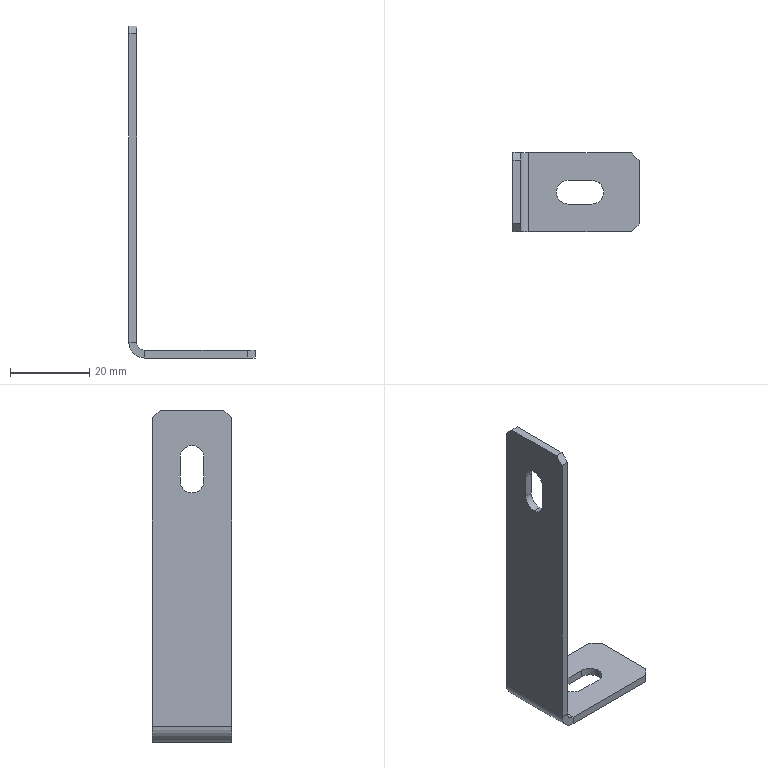Part | NX | features BREP 1 | 1 solid | 28 faces | box 32 x 20 x 84 mm | volume 4235 mm3 | plane 20 | cylinder 8 | commonest cylinder face diameters 6 x6 4 x1 8 x1
STEP:
#1=CARTESIAN_POINT('',(-2.,10.,-2.));
#2=VERTEX_POINT('',#1);
#3=CARTESIAN_POINT('',(0.,8.,-2.));
#4=VERTEX_POINT('',#3);
#5=CARTESIAN_POINT('',(0.,8.,-2.));
#6=DIRECTION('',(0.7071,-0.7071,0.));
#7=VECTOR('',#6,1000.);
#8=LINE('',#5,#7);
#9=EDGE_CURVE('',#2,#4,#8,.T.);
#10=ORIENTED_EDGE('',*,*,#9,.F.);
#11=CARTESIAN_POINT('',(-2.,10.,0.));
#12=VERTEX_POINT('',#11);
#13=CARTESIAN_POINT('',(-2.,10.,-2.));
#14=DIRECTION('',(0.,0.,-1.));
#15=VECTOR('',#14,1000.);
#16=LINE('',#13,#15);
#17=EDGE_CURVE('',#12,#2,#16,.T.);
#18=ORIENTED_EDGE('',*,*,#17,.F.);
#19=CARTESIAN_POINT('',(0.,8.,0.));
#20=VERTEX_POINT('',#19);
#21=CARTESIAN_POINT('',(-1.,9.,0.));
#22=DIRECTION('',(-0.7071,0.7071,0.));
#23=VECTOR('',#22,1000.);
#24=LINE('',#21,#23);
#25=EDGE_CURVE('',#20,#12,#24,.T.);
#26=ORIENTED_EDGE('',*,*,#25,.F.);
#27=CARTESIAN_POINT('',(0.,8.,0.));
#28=DIRECTION('',(0.,0.,1.));
#29=VECTOR('',#28,1000.);
#30=LINE('',#27,#29);
#31=EDGE_CURVE('',#4,#20,#30,.T.);
#32=ORIENTED_EDGE('',*,*,#31,.F.);
#33=EDGE_LOOP('',(#10,#18,#26,#32));
#34=FACE_BOUND('',#33,.T.);
#35=CARTESIAN_POINT('',(0.,8.,-2.));
#36=DIRECTION('',(0.7071,0.7071,0.));
#37=DIRECTION('',(0.,0.,-1.));
#38=AXIS2_PLACEMENT_3D('',#35,#36,#37);
#39=PLANE('',#38);
#40=ADVANCED_FACE('',(#34),#39,.T.);
#41=CARTESIAN_POINT('',(-30.,10.,80.));
#42=VERTEX_POINT('',#41);
#43=CARTESIAN_POINT('',(-30.,8.,82.));
#44=VERTEX_POINT('',#43);
#45=CARTESIAN_POINT('',(-30.,50.,40.));
#46=DIRECTION('',(0.,-0.7071,0.7071));
#47=VECTOR('',#46,1000.);
#48=LINE('',#45,#47);
#49=EDGE_CURVE('',#42,#44,#48,.T.);
#50=ORIENTED_EDGE('',*,*,#49,.F.);
#51=CARTESIAN_POINT('',(-32.,10.,80.));
#52=VERTEX_POINT('',#51);
#53=CARTESIAN_POINT('',(-28.,10.,80.));
#54=DIRECTION('',(1.,0.,0.));
#55=VECTOR('',#54,1000.);
#56=LINE('',#53,#55);
#57=EDGE_CURVE('',#52,#42,#56,.T.);
#58=ORIENTED_EDGE('',*,*,#57,.F.);
#59=CARTESIAN_POINT('',(-32.,8.,82.));
#60=VERTEX_POINT('',#59);
#61=CARTESIAN_POINT('',(-32.,8.,82.));
#62=DIRECTION('',(0.,0.7071,-0.7071));
#63=VECTOR('',#62,1000.);
#64=LINE('',#61,#63);
#65=EDGE_CURVE('',#60,#52,#64,.T.);
#66=ORIENTED_EDGE('',*,*,#65,.F.);
#67=CARTESIAN_POINT('',(-30.,8.,82.));
#68=DIRECTION('',(-1.,0.,0.));
#69=VECTOR('',#68,1000.);
#70=LINE('',#67,#69);
#71=EDGE_CURVE('',#44,#60,#70,.T.);
#72=ORIENTED_EDGE('',*,*,#71,.F.);
#73=EDGE_LOOP('',(#50,#58,#66,#72));
#74=FACE_BOUND('',#73,.T.);
#75=CARTESIAN_POINT('',(-30.,8.,82.));
#76=DIRECTION('',(0.,-0.7071,-0.7071));
#77=DIRECTION('',(-1.,0.,0.));
#78=AXIS2_PLACEMENT_3D('',#75,#76,#77);
#79=PLANE('',#78);
#80=ADVANCED_FACE('',(#74),#79,.F.);
#81=CARTESIAN_POINT('',(0.,-8.,-2.));
#82=VERTEX_POINT('',#81);
#83=CARTESIAN_POINT('',(-2.,-10.,-2.));
#84=VERTEX_POINT('',#83);
#85=CARTESIAN_POINT('',(-2.,-10.,-2.));
#86=DIRECTION('',(-0.7071,-0.7071,0.));
#87=VECTOR('',#86,1000.);
#88=LINE('',#85,#87);
#89=EDGE_CURVE('',#82,#84,#88,.T.);
#90=ORIENTED_EDGE('',*,*,#89,.F.);
#91=CARTESIAN_POINT('',(0.,-8.,0.));
#92=VERTEX_POINT('',#91);
#93=CARTESIAN_POINT('',(0.,-8.,-2.));
#94=DIRECTION('',(0.,0.,-1.));
#95=VECTOR('',#94,1000.);
#96=LINE('',#93,#95);
#97=EDGE_CURVE('',#92,#82,#96,.T.);
#98=ORIENTED_EDGE('',*,*,#97,.F.);
#99=CARTESIAN_POINT('',(-2.,-10.,0.));
#100=VERTEX_POINT('',#99);
#101=CARTESIAN_POINT('',(9.,1.,0.));
#102=DIRECTION('',(0.7071,0.7071,0.));
#103=VECTOR('',#102,1000.);
#104=LINE('',#101,#103);
#105=EDGE_CURVE('',#100,#92,#104,.T.);
#106=ORIENTED_EDGE('',*,*,#105,.F.);
#107=CARTESIAN_POINT('',(-2.,-10.,2.));
#108=DIRECTION('',(0.,0.,1.));
#109=VECTOR('',#108,1000.);
#110=LINE('',#107,#109);
#111=EDGE_CURVE('',#84,#100,#110,.T.);
#112=ORIENTED_EDGE('',*,*,#111,.F.);
#113=EDGE_LOOP('',(#90,#98,#106,#112));
#114=FACE_BOUND('',#113,.T.);
#115=CARTESIAN_POINT('',(-2.,-10.,2.));
#116=DIRECTION('',(-0.7071,0.7071,0.));
#117=DIRECTION('',(0.,0.,1.));
#118=AXIS2_PLACEMENT_3D('',#115,#116,#117);
#119=PLANE('',#118);
#120=ADVANCED_FACE('',(#114),#119,.F.);
#121=CARTESIAN_POINT('',(-30.,-8.,82.));
#122=VERTEX_POINT('',#121);
#123=CARTESIAN_POINT('',(-30.,-10.,80.));
#124=VERTEX_POINT('',#123);
#125=CARTESIAN_POINT('',(-30.,-40.,50.));
#126=DIRECTION('',(0.,-0.7071,-0.7071));
#127=VECTOR('',#126,1000.);
#128=LINE('',#125,#127);
#129=EDGE_CURVE('',#122,#124,#128,.T.);
#130=ORIENTED_EDGE('',*,*,#129,.F.);
#131=CARTESIAN_POINT('',(-32.,-8.,82.));
#132=VERTEX_POINT('',#131);
#133=CARTESIAN_POINT('',(-30.,-8.,82.));
#134=DIRECTION('',(1.,0.,0.));
#135=VECTOR('',#134,1000.);
#136=LINE('',#133,#135);
#137=EDGE_CURVE('',#132,#122,#136,.T.);
#138=ORIENTED_EDGE('',*,*,#137,.F.);
#139=CARTESIAN_POINT('',(-32.,-10.,80.));
#140=VERTEX_POINT('',#139);
#141=CARTESIAN_POINT('',(-32.,-10.,80.));
#142=DIRECTION('',(0.,0.7071,0.7071));
#143=VECTOR('',#142,1000.);
#144=LINE('',#141,#143);
#145=EDGE_CURVE('',#140,#132,#144,.T.);
#146=ORIENTED_EDGE('',*,*,#145,.F.);
#147=CARTESIAN_POINT('',(-28.,-10.,80.));
#148=DIRECTION('',(-1.,0.,0.));
#149=VECTOR('',#148,1000.);
#150=LINE('',#147,#149);
#151=EDGE_CURVE('',#124,#140,#150,.T.);
#152=ORIENTED_EDGE('',*,*,#151,.F.);
#153=EDGE_LOOP('',(#130,#138,#146,#152));
#154=FACE_BOUND('',#153,.T.);
#155=CARTESIAN_POINT('',(-28.,-10.,80.));
#156=DIRECTION('',(0.,0.7071,-0.7071));
#157=DIRECTION('',(-1.,0.,0.));
#158=AXIS2_PLACEMENT_3D('',#155,#156,#157);
#159=PLANE('',#158);
#160=ADVANCED_FACE('',(#154),#159,.F.);
#161=CARTESIAN_POINT('',(-18.,-3.,0.));
#162=VERTEX_POINT('',#161);
#163=CARTESIAN_POINT('',(-12.,-3.,0.));
#164=VERTEX_POINT('',#163);
#165=CARTESIAN_POINT('',(-18.,-3.,0.));
#166=DIRECTION('',(1.,0.,0.));
#167=VECTOR('',#166,1000.);
#168=LINE('',#165,#167);
#169=EDGE_CURVE('',#162,#164,#168,.T.);
#170=ORIENTED_EDGE('',*,*,#169,.T.);
#171=CARTESIAN_POINT('',(-12.,-3.,-2.));
#172=VERTEX_POINT('',#171);
#173=CARTESIAN_POINT('',(-12.,-3.,-2.));
#174=DIRECTION('',(0.,0.,1.));
#175=VECTOR('',#174,1000.);
#176=LINE('',#173,#175);
#177=EDGE_CURVE('',#172,#164,#176,.T.);
#178=ORIENTED_EDGE('',*,*,#177,.F.);
#179=CARTESIAN_POINT('',(-18.,-3.,-2.));
#180=VERTEX_POINT('',#179);
#181=CARTESIAN_POINT('',(-18.,-3.,-2.));
#182=DIRECTION('',(1.,0.,0.));
#183=VECTOR('',#182,1000.);
#184=LINE('',#181,#183);
#185=EDGE_CURVE('',#180,#172,#184,.T.);
#186=ORIENTED_EDGE('',*,*,#185,.F.);
#187=CARTESIAN_POINT('',(-18.,-3.,-2.));
#188=DIRECTION('',(0.,0.,1.));
#189=VECTOR('',#188,1000.);
#190=LINE('',#187,#189);
#191=EDGE_CURVE('',#180,#162,#190,.T.);
#192=ORIENTED_EDGE('',*,*,#191,.T.);
#193=EDGE_LOOP('',(#170,#178,#186,#192));
#194=FACE_BOUND('',#193,.T.);
#195=CARTESIAN_POINT('',(-18.,-3.,-2.));
#196=DIRECTION('',(0.,-1.,0.));
#197=DIRECTION('',(1.,0.,0.));
#198=AXIS2_PLACEMENT_3D('',#195,#196,#197);
#199=PLANE('',#198);
#200=ADVANCED_FACE('',(#194),#199,.F.);
#201=CARTESIAN_POINT('',(-9.,0.,-2.));
#202=VERTEX_POINT('',#201);
#203=CARTESIAN_POINT('',(-9.,0.,0.));
#204=VERTEX_POINT('',#203);
#205=CARTESIAN_POINT('',(-9.,0.,-2.));
#206=DIRECTION('',(0.,0.,1.));
#207=VECTOR('',#206,1000.);
#208=LINE('',#205,#207);
#209=EDGE_CURVE('',#202,#204,#208,.T.);
#210=ORIENTED_EDGE('',*,*,#209,.F.);
#211=CARTESIAN_POINT('',(-12.,0.,-2.));
#212=DIRECTION('',(0.,0.,1.));
#213=DIRECTION('',(1.,0.,0.));
#214=AXIS2_PLACEMENT_3D('',#211,#212,#213);
#215=CIRCLE('',#214,3.);
#216=EDGE_CURVE('',#172,#202,#215,.T.);
#217=ORIENTED_EDGE('',*,*,#216,.F.);
#218=ORIENTED_EDGE('',*,*,#177,.T.);
#219=CARTESIAN_POINT('',(-12.,0.,0.));
#220=DIRECTION('',(0.,0.,1.));
#221=DIRECTION('',(1.,0.,0.));
#222=AXIS2_PLACEMENT_3D('',#219,#220,#221);
#223=CIRCLE('',#222,3.);
#224=EDGE_CURVE('',#164,#204,#223,.T.);
#225=ORIENTED_EDGE('',*,*,#224,.T.);
#226=EDGE_LOOP('',(#210,#217,#218,#225));
#227=FACE_BOUND('',#226,.T.);
#228=CARTESIAN_POINT('',(-12.,0.,-2.));
#229=DIRECTION('',(0.,0.,1.));
#230=DIRECTION('',(1.,0.,0.));
#231=AXIS2_PLACEMENT_3D('',#228,#229,#230);
#232=CYLINDRICAL_SURFACE('',#231,3.);
#233=ADVANCED_FACE('',(#227),#232,.F.);
#234=CARTESIAN_POINT('',(-12.,3.,0.));
#235=VERTEX_POINT('',#234);
#236=CARTESIAN_POINT('',(-18.,3.,0.));
#237=VERTEX_POINT('',#236);
#238=CARTESIAN_POINT('',(-18.,3.,0.));
#239=DIRECTION('',(-1.,0.,0.));
#240=VECTOR('',#239,1000.);
#241=LINE('',#238,#240);
#242=EDGE_CURVE('',#235,#237,#241,.T.);
#243=ORIENTED_EDGE('',*,*,#242,.T.);
#244=CARTESIAN_POINT('',(-18.,3.,-2.));
#245=VERTEX_POINT('',#244);
#246=CARTESIAN_POINT('',(-18.,3.,-2.));
#247=DIRECTION('',(0.,0.,1.));
#248=VECTOR('',#247,1000.);
#249=LINE('',#246,#248);
#250=EDGE_CURVE('',#245,#237,#249,.T.);
#251=ORIENTED_EDGE('',*,*,#250,.F.);
#252=CARTESIAN_POINT('',(-12.,3.,-2.));
#253=VERTEX_POINT('',#252);
#254=CARTESIAN_POINT('',(-18.,3.,-2.));
#255=DIRECTION('',(-1.,0.,0.));
#256=VECTOR('',#255,1000.);
#257=LINE('',#254,#256);
#258=EDGE_CURVE('',#253,#245,#257,.T.);
#259=ORIENTED_EDGE('',*,*,#258,.F.);
#260=CARTESIAN_POINT('',(-12.,3.,-2.));
#261=DIRECTION('',(0.,0.,1.));
#262=VECTOR('',#261,1000.);
#263=LINE('',#260,#262);
#264=EDGE_CURVE('',#253,#235,#263,.T.);
#265=ORIENTED_EDGE('',*,*,#264,.T.);
#266=EDGE_LOOP('',(#243,#251,#259,#265));
#267=FACE_BOUND('',#266,.T.);
#268=CARTESIAN_POINT('',(-18.,3.,-2.));
#269=DIRECTION('',(0.,1.,0.));
#270=DIRECTION('',(-1.,0.,0.));
#271=AXIS2_PLACEMENT_3D('',#268,#269,#270);
#272=PLANE('',#271);
#273=ADVANCED_FACE('',(#267),#272,.F.);
#274=CARTESIAN_POINT('',(-18.,0.,0.));
#275=DIRECTION('',(0.,0.,1.));
#276=DIRECTION('',(1.,0.,0.));
#277=AXIS2_PLACEMENT_3D('',#274,#275,#276);
#278=CIRCLE('',#277,3.);
#279=EDGE_CURVE('',#237,#162,#278,.T.);
#280=ORIENTED_EDGE('',*,*,#279,.T.);
#281=ORIENTED_EDGE('',*,*,#191,.F.);
#282=CARTESIAN_POINT('',(-18.,0.,-2.));
#283=DIRECTION('',(0.,0.,1.));
#284=DIRECTION('',(1.,0.,0.));
#285=AXIS2_PLACEMENT_3D('',#282,#283,#284);
#286=CIRCLE('',#285,3.);
#287=EDGE_CURVE('',#245,#180,#286,.T.);
#288=ORIENTED_EDGE('',*,*,#287,.F.);
#289=ORIENTED_EDGE('',*,*,#250,.T.);
#290=EDGE_LOOP('',(#280,#281,#288,#289));
#291=FACE_BOUND('',#290,.T.);
#292=CARTESIAN_POINT('',(-18.,0.,-2.));
#293=DIRECTION('',(0.,0.,1.));
#294=DIRECTION('',(1.,0.,0.));
#295=AXIS2_PLACEMENT_3D('',#292,#293,#294);
#296=CYLINDRICAL_SURFACE('',#295,3.);
#297=ADVANCED_FACE('',(#291),#296,.F.);
#298=CARTESIAN_POINT('',(-30.,-3.,70.));
#299=VERTEX_POINT('',#298);
#300=CARTESIAN_POINT('',(-30.,-3.,64.));
#301=VERTEX_POINT('',#300);
#302=CARTESIAN_POINT('',(-30.,-3.,70.));
#303=DIRECTION('',(0.,0.,-1.));
#304=VECTOR('',#303,1000.);
#305=LINE('',#302,#304);
#306=EDGE_CURVE('',#299,#301,#305,.T.);
#307=ORIENTED_EDGE('',*,*,#306,.T.);
#308=CARTESIAN_POINT('',(-32.,-3.,64.));
#309=VERTEX_POINT('',#308);
#310=CARTESIAN_POINT('',(-32.,-3.,64.));
#311=DIRECTION('',(1.,0.,0.));
#312=VECTOR('',#311,1000.);
#313=LINE('',#310,#312);
#314=EDGE_CURVE('',#309,#301,#313,.T.);
#315=ORIENTED_EDGE('',*,*,#314,.F.);
#316=CARTESIAN_POINT('',(-32.,-3.,70.));
#317=VERTEX_POINT('',#316);
#318=CARTESIAN_POINT('',(-32.,-3.,70.));
#319=DIRECTION('',(0.,0.,-1.));
#320=VECTOR('',#319,1000.);
#321=LINE('',#318,#320);
#322=EDGE_CURVE('',#317,#309,#321,.T.);
#323=ORIENTED_EDGE('',*,*,#322,.F.);
#324=CARTESIAN_POINT('',(-32.,-3.,70.));
#325=DIRECTION('',(1.,0.,0.));
#326=VECTOR('',#325,1000.);
#327=LINE('',#324,#326);
#328=EDGE_CURVE('',#317,#299,#327,.T.);
#329=ORIENTED_EDGE('',*,*,#328,.T.);
#330=EDGE_LOOP('',(#307,#315,#323,#329));
#331=FACE_BOUND('',#330,.T.);
#332=CARTESIAN_POINT('',(-32.,-3.,70.));
#333=DIRECTION('',(0.,-1.,0.));
#334=DIRECTION('',(0.,0.,-1.));
#335=AXIS2_PLACEMENT_3D('',#332,#333,#334);
#336=PLANE('',#335);
#337=ADVANCED_FACE('',(#331),#336,.F.);
#338=CARTESIAN_POINT('',(-32.,0.,61.));
#339=VERTEX_POINT('',#338);
#340=CARTESIAN_POINT('',(-30.,0.,61.));
#341=VERTEX_POINT('',#340);
#342=CARTESIAN_POINT('',(-32.,0.,61.));
#343=DIRECTION('',(1.,0.,0.));
#344=VECTOR('',#343,1000.);
#345=LINE('',#342,#344);
#346=EDGE_CURVE('',#339,#341,#345,.T.);
#347=ORIENTED_EDGE('',*,*,#346,.F.);
#348=CARTESIAN_POINT('',(-32.,0.,64.));
#349=DIRECTION('',(1.,0.,0.));
#350=DIRECTION('',(0.,0.,-1.));
#351=AXIS2_PLACEMENT_3D('',#348,#349,#350);
#352=CIRCLE('',#351,3.);
#353=EDGE_CURVE('',#309,#339,#352,.T.);
#354=ORIENTED_EDGE('',*,*,#353,.F.);
#355=ORIENTED_EDGE('',*,*,#314,.T.);
#356=CARTESIAN_POINT('',(-30.,0.,64.));
#357=DIRECTION('',(1.,0.,0.));
#358=DIRECTION('',(0.,0.,-1.));
#359=AXIS2_PLACEMENT_3D('',#356,#357,#358);
#360=CIRCLE('',#359,3.);
#361=EDGE_CURVE('',#301,#341,#360,.T.);
#362=ORIENTED_EDGE('',*,*,#361,.T.);
#363=EDGE_LOOP('',(#347,#354,#355,#362));
#364=FACE_BOUND('',#363,.T.);
#365=CARTESIAN_POINT('',(-32.,0.,64.));
#366=DIRECTION('',(1.,0.,0.));
#367=DIRECTION('',(0.,0.,-1.));
#368=AXIS2_PLACEMENT_3D('',#365,#366,#367);
#369=CYLINDRICAL_SURFACE('',#368,3.);
#370=ADVANCED_FACE('',(#364),#369,.F.);
#371=CARTESIAN_POINT('',(-30.,3.,64.));
#372=VERTEX_POINT('',#371);
#373=CARTESIAN_POINT('',(-30.,3.,70.));
#374=VERTEX_POINT('',#373);
#375=CARTESIAN_POINT('',(-30.,3.,70.));
#376=DIRECTION('',(0.,0.,1.));
#377=VECTOR('',#376,1000.);
#378=LINE('',#375,#377);
#379=EDGE_CURVE('',#372,#374,#378,.T.);
#380=ORIENTED_EDGE('',*,*,#379,.T.);
#381=CARTESIAN_POINT('',(-32.,3.,70.));
#382=VERTEX_POINT('',#381);
#383=CARTESIAN_POINT('',(-32.,3.,70.));
#384=DIRECTION('',(1.,0.,0.));
#385=VECTOR('',#384,1000.);
#386=LINE('',#383,#385);
#387=EDGE_CURVE('',#382,#374,#386,.T.);
#388=ORIENTED_EDGE('',*,*,#387,.F.);
#389=CARTESIAN_POINT('',(-32.,3.,64.));
#390=VERTEX_POINT('',#389);
#391=CARTESIAN_POINT('',(-32.,3.,70.));
#392=DIRECTION('',(0.,0.,1.));
#393=VECTOR('',#392,1000.);
#394=LINE('',#391,#393);
#395=EDGE_CURVE('',#390,#382,#394,.T.);
#396=ORIENTED_EDGE('',*,*,#395,.F.);
#397=CARTESIAN_POINT('',(-32.,3.,64.));
#398=DIRECTION('',(1.,0.,0.));
#399=VECTOR('',#398,1000.);
#400=LINE('',#397,#399);
#401=EDGE_CURVE('',#390,#372,#400,.T.);
#402=ORIENTED_EDGE('',*,*,#401,.T.);
#403=EDGE_LOOP('',(#380,#388,#396,#402));
#404=FACE_BOUND('',#403,.T.);
#405=CARTESIAN_POINT('',(-32.,3.,70.));
#406=DIRECTION('',(0.,1.,0.));
#407=DIRECTION('',(0.,0.,1.));
#408=AXIS2_PLACEMENT_3D('',#405,#406,#407);
#409=PLANE('',#408);
#410=ADVANCED_FACE('',(#404),#409,.F.);
#411=CARTESIAN_POINT('',(-30.,0.,70.));
#412=DIRECTION('',(1.,0.,0.));
#413=DIRECTION('',(0.,0.,-1.));
#414=AXIS2_PLACEMENT_3D('',#411,#412,#413);
#415=CIRCLE('',#414,3.);
#416=EDGE_CURVE('',#374,#299,#415,.T.);
#417=ORIENTED_EDGE('',*,*,#416,.T.);
#418=ORIENTED_EDGE('',*,*,#328,.F.);
#419=CARTESIAN_POINT('',(-32.,0.,70.));
#420=DIRECTION('',(1.,0.,0.));
#421=DIRECTION('',(0.,0.,-1.));
#422=AXIS2_PLACEMENT_3D('',#419,#420,#421);
#423=CIRCLE('',#422,3.);
#424=EDGE_CURVE('',#382,#317,#423,.T.);
#425=ORIENTED_EDGE('',*,*,#424,.F.);
#426=ORIENTED_EDGE('',*,*,#387,.T.);
#427=EDGE_LOOP('',(#417,#418,#425,#426));
#428=FACE_BOUND('',#427,.T.);
#429=CARTESIAN_POINT('',(-32.,0.,70.));
#430=DIRECTION('',(1.,0.,0.));
#431=DIRECTION('',(0.,0.,-1.));
#432=AXIS2_PLACEMENT_3D('',#429,#430,#431);
#433=CYLINDRICAL_SURFACE('',#432,3.);
#434=ADVANCED_FACE('',(#428),#433,.F.);
#435=CARTESIAN_POINT('',(-30.,-10.,2.));
#436=VERTEX_POINT('',#435);
#437=CARTESIAN_POINT('',(-30.,-10.,0.));
#438=DIRECTION('',(0.,0.,1.));
#439=VECTOR('',#438,1000.);
#440=LINE('',#437,#439);
#441=EDGE_CURVE('',#436,#124,#440,.T.);
#442=ORIENTED_EDGE('',*,*,#441,.T.);
#443=ORIENTED_EDGE('',*,*,#151,.T.);
#444=CARTESIAN_POINT('',(-32.,-10.,2.));
#445=VERTEX_POINT('',#444);
#446=CARTESIAN_POINT('',(-32.,-10.,0.));
#447=DIRECTION('',(0.,0.,1.));
#448=VECTOR('',#447,1000.);
#449=LINE('',#446,#448);
#450=EDGE_CURVE('',#445,#140,#449,.T.);
#451=ORIENTED_EDGE('',*,*,#450,.F.);
#452=CARTESIAN_POINT('',(-32.,-10.,2.));
#453=DIRECTION('',(1.,0.,0.));
#454=VECTOR('',#453,1000.);
#455=LINE('',#452,#454);
#456=EDGE_CURVE('',#445,#436,#455,.T.);
#457=ORIENTED_EDGE('',*,*,#456,.T.);
#458=EDGE_LOOP('',(#442,#443,#451,#457));
#459=FACE_BOUND('',#458,.T.);
#460=CARTESIAN_POINT('',(-28.,-10.,2.));
#461=DIRECTION('',(0.,-1.,0.));
#462=DIRECTION('',(-1.,0.,0.));
#463=AXIS2_PLACEMENT_3D('',#460,#461,#462);
#464=PLANE('',#463);
#465=ADVANCED_FACE('',(#459),#464,.T.);
#466=CARTESIAN_POINT('',(-28.,10.,0.));
#467=VERTEX_POINT('',#466);
#468=CARTESIAN_POINT('',(0.,10.,0.));
#469=DIRECTION('',(-1.,0.,0.));
#470=VECTOR('',#469,1000.);
#471=LINE('',#468,#470);
#472=EDGE_CURVE('',#12,#467,#471,.T.);
#473=ORIENTED_EDGE('',*,*,#472,.F.);
#474=ORIENTED_EDGE('',*,*,#17,.T.);
#475=CARTESIAN_POINT('',(-28.,10.,-2.));
#476=VERTEX_POINT('',#475);
#477=CARTESIAN_POINT('',(0.,10.,-2.));
#478=DIRECTION('',(-1.,0.,0.));
#479=VECTOR('',#478,1000.);
#480=LINE('',#477,#479);
#481=EDGE_CURVE('',#2,#476,#480,.T.);
#482=ORIENTED_EDGE('',*,*,#481,.T.);
#483=CARTESIAN_POINT('',(-28.,10.,-2.));
#484=DIRECTION('',(0.,0.,1.));
#485=VECTOR('',#484,1000.);
#486=LINE('',#483,#485);
#487=EDGE_CURVE('',#476,#467,#486,.T.);
#488=ORIENTED_EDGE('',*,*,#487,.T.);
#489=EDGE_LOOP('',(#473,#474,#482,#488));
#490=FACE_BOUND('',#489,.T.);
#491=CARTESIAN_POINT('',(-28.,10.,2.));
#492=DIRECTION('',(0.,-1.,0.));
#493=DIRECTION('',(-1.,0.,0.));
#494=AXIS2_PLACEMENT_3D('',#491,#492,#493);
#495=PLANE('',#494);
#496=ADVANCED_FACE('',(#490),#495,.F.);
#497=CARTESIAN_POINT('',(-28.,-10.,-2.));
#498=VERTEX_POINT('',#497);
#499=CARTESIAN_POINT('',(-28.,-10.,2.));
#500=DIRECTION('',(0.,1.,0.));
#501=DIRECTION('',(1.,0.,0.));
#502=AXIS2_PLACEMENT_3D('',#499,#500,#501);
#503=CIRCLE('',#502,4.);
#504=EDGE_CURVE('',#498,#445,#503,.T.);
#505=ORIENTED_EDGE('',*,*,#504,.T.);
#506=CARTESIAN_POINT('',(-32.,10.,2.));
#507=VERTEX_POINT('',#506);
#508=CARTESIAN_POINT('',(-32.,10.,2.));
#509=DIRECTION('',(0.,-1.,0.));
#510=VECTOR('',#509,1000.);
#511=LINE('',#508,#510);
#512=EDGE_CURVE('',#507,#445,#511,.T.);
#513=ORIENTED_EDGE('',*,*,#512,.F.);
#514=CARTESIAN_POINT('',(-28.,10.,2.));
#515=DIRECTION('',(0.,1.,0.));
#516=DIRECTION('',(1.,0.,0.));
#517=AXIS2_PLACEMENT_3D('',#514,#515,#516);
#518=CIRCLE('',#517,4.);
#519=EDGE_CURVE('',#476,#507,#518,.T.);
#520=ORIENTED_EDGE('',*,*,#519,.F.);
#521=CARTESIAN_POINT('',(-28.,10.,-2.));
#522=DIRECTION('',(0.,-1.,0.));
#523=VECTOR('',#522,1000.);
#524=LINE('',#521,#523);
#525=EDGE_CURVE('',#476,#498,#524,.T.);
#526=ORIENTED_EDGE('',*,*,#525,.T.);
#527=EDGE_LOOP('',(#505,#513,#520,#526));
#528=FACE_BOUND('',#527,.T.);
#529=CARTESIAN_POINT('',(-28.,10.,2.));
#530=DIRECTION('',(0.,-1.,0.));
#531=DIRECTION('',(0.,0.,-1.));
#532=AXIS2_PLACEMENT_3D('',#529,#530,#531);
#533=CYLINDRICAL_SURFACE('',#532,4.);
#534=ADVANCED_FACE('',(#528),#533,.T.);
#535=CARTESIAN_POINT('',(0.,10.,-2.));
#536=DIRECTION('',(0.,-1.,0.));
#537=VECTOR('',#536,1000.);
#538=LINE('',#535,#537);
#539=EDGE_CURVE('',#4,#82,#538,.T.);
#540=ORIENTED_EDGE('',*,*,#539,.T.);
#541=ORIENTED_EDGE('',*,*,#89,.T.);
#542=CARTESIAN_POINT('',(0.,-10.,-2.));
#543=DIRECTION('',(-1.,0.,0.));
#544=VECTOR('',#543,1000.);
#545=LINE('',#542,#544);
#546=EDGE_CURVE('',#84,#498,#545,.T.);
#547=ORIENTED_EDGE('',*,*,#546,.T.);
#548=ORIENTED_EDGE('',*,*,#525,.F.);
#549=ORIENTED_EDGE('',*,*,#481,.F.);
#550=ORIENTED_EDGE('',*,*,#9,.T.);
#551=EDGE_LOOP('',(#540,#541,#547,#548,#549,#550));
#552=FACE_BOUND('',#551,.T.);
#553=ORIENTED_EDGE('',*,*,#258,.T.);
#554=ORIENTED_EDGE('',*,*,#287,.T.);
#555=ORIENTED_EDGE('',*,*,#185,.T.);
#556=ORIENTED_EDGE('',*,*,#216,.T.);
#557=CARTESIAN_POINT('',(-12.,0.,-2.));
#558=DIRECTION('',(0.,0.,1.));
#559=DIRECTION('',(1.,0.,0.));
#560=AXIS2_PLACEMENT_3D('',#557,#558,#559);
#561=CIRCLE('',#560,3.);
#562=EDGE_CURVE('',#202,#253,#561,.T.);
#563=ORIENTED_EDGE('',*,*,#562,.T.);
#564=EDGE_LOOP('',(#553,#554,#555,#556,#563));
#565=FACE_BOUND('',#564,.T.);
#566=CARTESIAN_POINT('',(0.,10.,-2.));
#567=DIRECTION('',(0.,0.,1.));
#568=DIRECTION('',(1.,0.,0.));
#569=AXIS2_PLACEMENT_3D('',#566,#567,#568);
#570=PLANE('',#569);
#571=ADVANCED_FACE('',(#552,#565),#570,.F.);
#572=CARTESIAN_POINT('',(0.,10.,0.));
#573=DIRECTION('',(0.,-1.,0.));
#574=VECTOR('',#573,1000.);
#575=LINE('',#572,#574);
#576=EDGE_CURVE('',#20,#92,#575,.T.);
#577=ORIENTED_EDGE('',*,*,#576,.T.);
#578=ORIENTED_EDGE('',*,*,#97,.T.);
#579=ORIENTED_EDGE('',*,*,#539,.F.);
#580=ORIENTED_EDGE('',*,*,#31,.T.);
#581=EDGE_LOOP('',(#577,#578,#579,#580));
#582=FACE_BOUND('',#581,.T.);
#583=CARTESIAN_POINT('',(0.,10.,-2.));
#584=DIRECTION('',(1.,0.,0.));
#585=DIRECTION('',(0.,0.,-1.));
#586=AXIS2_PLACEMENT_3D('',#583,#584,#585);
#587=PLANE('',#586);
#588=ADVANCED_FACE('',(#582),#587,.T.);
#589=CARTESIAN_POINT('',(-28.,-10.,0.));
#590=VERTEX_POINT('',#589);
#591=CARTESIAN_POINT('',(0.,-10.,0.));
#592=DIRECTION('',(-1.,0.,0.));
#593=VECTOR('',#592,1000.);
#594=LINE('',#591,#593);
#595=EDGE_CURVE('',#100,#590,#594,.T.);
#596=ORIENTED_EDGE('',*,*,#595,.F.);
#597=ORIENTED_EDGE('',*,*,#105,.T.);
#598=ORIENTED_EDGE('',*,*,#576,.F.);
#599=ORIENTED_EDGE('',*,*,#25,.T.);
#600=ORIENTED_EDGE('',*,*,#472,.T.);
#601=CARTESIAN_POINT('',(-28.,10.,0.));
#602=DIRECTION('',(0.,-1.,0.));
#603=VECTOR('',#602,1000.);
#604=LINE('',#601,#603);
#605=EDGE_CURVE('',#467,#590,#604,.T.);
#606=ORIENTED_EDGE('',*,*,#605,.T.);
#607=EDGE_LOOP('',(#596,#597,#598,#599,#600,#606));
#608=FACE_BOUND('',#607,.T.);
#609=ORIENTED_EDGE('',*,*,#279,.F.);
#610=ORIENTED_EDGE('',*,*,#242,.F.);
#611=CARTESIAN_POINT('',(-12.,0.,0.));
#612=DIRECTION('',(0.,0.,1.));
#613=DIRECTION('',(1.,0.,0.));
#614=AXIS2_PLACEMENT_3D('',#611,#612,#613);
#615=CIRCLE('',#614,3.);
#616=EDGE_CURVE('',#204,#235,#615,.T.);
#617=ORIENTED_EDGE('',*,*,#616,.F.);
#618=ORIENTED_EDGE('',*,*,#224,.F.);
#619=ORIENTED_EDGE('',*,*,#169,.F.);
#620=EDGE_LOOP('',(#609,#610,#617,#618,#619));
#621=FACE_BOUND('',#620,.T.);
#622=CARTESIAN_POINT('',(0.,10.,0.));
#623=DIRECTION('',(0.,0.,1.));
#624=DIRECTION('',(1.,0.,0.));
#625=AXIS2_PLACEMENT_3D('',#622,#623,#624);
#626=PLANE('',#625);
#627=ADVANCED_FACE('',(#608,#621),#626,.T.);
#628=CARTESIAN_POINT('',(-28.,-10.,2.));
#629=DIRECTION('',(0.,1.,0.));
#630=DIRECTION('',(0.,0.,-1.));
#631=AXIS2_PLACEMENT_3D('',#628,#629,#630);
#632=CIRCLE('',#631,2.);
#633=EDGE_CURVE('',#590,#436,#632,.T.);
#634=ORIENTED_EDGE('',*,*,#633,.F.);
#635=ORIENTED_EDGE('',*,*,#605,.F.);
#636=CARTESIAN_POINT('',(-30.,10.,2.));
#637=VERTEX_POINT('',#636);
#638=CARTESIAN_POINT('',(-28.,10.,2.));
#639=DIRECTION('',(0.,1.,0.));
#640=DIRECTION('',(0.,0.,-1.));
#641=AXIS2_PLACEMENT_3D('',#638,#639,#640);
#642=CIRCLE('',#641,2.);
#643=EDGE_CURVE('',#467,#637,#642,.T.);
#644=ORIENTED_EDGE('',*,*,#643,.T.);
#645=CARTESIAN_POINT('',(-30.,10.,2.));
#646=DIRECTION('',(0.,-1.,0.));
#647=VECTOR('',#646,1000.);
#648=LINE('',#645,#647);
#649=EDGE_CURVE('',#637,#436,#648,.T.);
#650=ORIENTED_EDGE('',*,*,#649,.T.);
#651=EDGE_LOOP('',(#634,#635,#644,#650));
#652=FACE_BOUND('',#651,.T.);
#653=CARTESIAN_POINT('',(-28.,10.,2.));
#654=DIRECTION('',(0.,-1.,0.));
#655=DIRECTION('',(0.,0.,-1.));
#656=AXIS2_PLACEMENT_3D('',#653,#654,#655);
#657=CYLINDRICAL_SURFACE('',#656,2.);
#658=ADVANCED_FACE('',(#652),#657,.F.);
#659=CARTESIAN_POINT('',(-30.,10.,82.));
#660=DIRECTION('',(0.,-1.,0.));
#661=VECTOR('',#660,1000.);
#662=LINE('',#659,#661);
#663=EDGE_CURVE('',#44,#122,#662,.T.);
#664=ORIENTED_EDGE('',*,*,#663,.T.);
#665=ORIENTED_EDGE('',*,*,#129,.T.);
#666=ORIENTED_EDGE('',*,*,#441,.F.);
#667=ORIENTED_EDGE('',*,*,#649,.F.);
#668=CARTESIAN_POINT('',(-30.,10.,0.));
#669=DIRECTION('',(0.,0.,1.));
#670=VECTOR('',#669,1000.);
#671=LINE('',#668,#670);
#672=EDGE_CURVE('',#637,#42,#671,.T.);
#673=ORIENTED_EDGE('',*,*,#672,.T.);
#674=ORIENTED_EDGE('',*,*,#49,.T.);
#675=EDGE_LOOP('',(#664,#665,#666,#667,#673,#674));
#676=FACE_BOUND('',#675,.T.);
#677=ORIENTED_EDGE('',*,*,#416,.F.);
#678=ORIENTED_EDGE('',*,*,#379,.F.);
#679=CARTESIAN_POINT('',(-30.,0.,64.));
#680=DIRECTION('',(1.,0.,0.));
#681=DIRECTION('',(0.,0.,-1.));
#682=AXIS2_PLACEMENT_3D('',#679,#680,#681);
#683=CIRCLE('',#682,3.);
#684=EDGE_CURVE('',#341,#372,#683,.T.);
#685=ORIENTED_EDGE('',*,*,#684,.F.);
#686=ORIENTED_EDGE('',*,*,#361,.F.);
#687=ORIENTED_EDGE('',*,*,#306,.F.);
#688=EDGE_LOOP('',(#677,#678,#685,#686,#687));
#689=FACE_BOUND('',#688,.T.);
#690=CARTESIAN_POINT('',(-30.,10.,0.));
#691=DIRECTION('',(1.,0.,0.));
#692=DIRECTION('',(0.,0.,-1.));
#693=AXIS2_PLACEMENT_3D('',#690,#691,#692);
#694=PLANE('',#693);
#695=ADVANCED_FACE('',(#676,#689),#694,.T.);
#696=CARTESIAN_POINT('',(-32.,10.,82.));
#697=DIRECTION('',(0.,-1.,0.));
#698=VECTOR('',#697,1000.);
#699=LINE('',#696,#698);
#700=EDGE_CURVE('',#60,#132,#699,.T.);
#701=ORIENTED_EDGE('',*,*,#700,.T.);
#702=ORIENTED_EDGE('',*,*,#137,.T.);
#703=ORIENTED_EDGE('',*,*,#663,.F.);
#704=ORIENTED_EDGE('',*,*,#71,.T.);
#705=EDGE_LOOP('',(#701,#702,#703,#704));
#706=FACE_BOUND('',#705,.T.);
#707=CARTESIAN_POINT('',(-30.,10.,82.));
#708=DIRECTION('',(0.,0.,1.));
#709=DIRECTION('',(1.,0.,0.));
#710=AXIS2_PLACEMENT_3D('',#707,#708,#709);
#711=PLANE('',#710);
#712=ADVANCED_FACE('',(#706),#711,.T.);
#713=ORIENTED_EDGE('',*,*,#450,.T.);
#714=ORIENTED_EDGE('',*,*,#145,.T.);
#715=ORIENTED_EDGE('',*,*,#700,.F.);
#716=ORIENTED_EDGE('',*,*,#65,.T.);
#717=CARTESIAN_POINT('',(-32.,10.,0.));
#718=DIRECTION('',(0.,0.,1.));
#719=VECTOR('',#718,1000.);
#720=LINE('',#717,#719);
#721=EDGE_CURVE('',#507,#52,#720,.T.);
#722=ORIENTED_EDGE('',*,*,#721,.F.);
#723=ORIENTED_EDGE('',*,*,#512,.T.);
#724=EDGE_LOOP('',(#713,#714,#715,#716,#722,#723));
#725=FACE_BOUND('',#724,.T.);
#726=ORIENTED_EDGE('',*,*,#395,.T.);
#727=ORIENTED_EDGE('',*,*,#424,.T.);
#728=ORIENTED_EDGE('',*,*,#322,.T.);
#729=ORIENTED_EDGE('',*,*,#353,.T.);
#730=CARTESIAN_POINT('',(-32.,0.,64.));
#731=DIRECTION('',(1.,0.,0.));
#732=DIRECTION('',(0.,0.,-1.));
#733=AXIS2_PLACEMENT_3D('',#730,#731,#732);
#734=CIRCLE('',#733,3.);
#735=EDGE_CURVE('',#339,#390,#734,.T.);
#736=ORIENTED_EDGE('',*,*,#735,.T.);
#737=EDGE_LOOP('',(#726,#727,#728,#729,#736));
#738=FACE_BOUND('',#737,.T.);
#739=CARTESIAN_POINT('',(-32.,10.,0.));
#740=DIRECTION('',(1.,0.,0.));
#741=DIRECTION('',(0.,0.,-1.));
#742=AXIS2_PLACEMENT_3D('',#739,#740,#741);
#743=PLANE('',#742);
#744=ADVANCED_FACE('',(#725,#738),#743,.F.);
#745=ORIENTED_EDGE('',*,*,#546,.F.);
#746=ORIENTED_EDGE('',*,*,#111,.T.);
#747=ORIENTED_EDGE('',*,*,#595,.T.);
#748=CARTESIAN_POINT('',(-28.,-10.,0.));
#749=DIRECTION('',(0.,0.,-1.));
#750=VECTOR('',#749,1000.);
#751=LINE('',#748,#750);
#752=EDGE_CURVE('',#590,#498,#751,.T.);
#753=ORIENTED_EDGE('',*,*,#752,.T.);
#754=EDGE_LOOP('',(#745,#746,#747,#753));
#755=FACE_BOUND('',#754,.T.);
#756=CARTESIAN_POINT('',(-32.,-10.,2.));
#757=DIRECTION('',(0.,-1.,0.));
#758=DIRECTION('',(0.,0.,-1.));
#759=AXIS2_PLACEMENT_3D('',#756,#757,#758);
#760=PLANE('',#759);
#761=ADVANCED_FACE('',(#755),#760,.T.);
#762=ORIENTED_EDGE('',*,*,#752,.F.);
#763=ORIENTED_EDGE('',*,*,#633,.T.);
#764=ORIENTED_EDGE('',*,*,#456,.F.);
#765=ORIENTED_EDGE('',*,*,#504,.F.);
#766=EDGE_LOOP('',(#762,#763,#764,#765));
#767=FACE_BOUND('',#766,.T.);
#768=CARTESIAN_POINT('',(-28.,-10.,0.));
#769=DIRECTION('',(0.,-1.,0.));
#770=DIRECTION('',(0.,0.,-1.));
#771=AXIS2_PLACEMENT_3D('',#768,#769,#770);
#772=PLANE('',#771);
#773=ADVANCED_FACE('',(#767),#772,.T.);
#774=ORIENTED_EDGE('',*,*,#721,.T.);
#775=ORIENTED_EDGE('',*,*,#57,.T.);
#776=ORIENTED_EDGE('',*,*,#672,.F.);
#777=CARTESIAN_POINT('',(-30.,10.,2.));
#778=DIRECTION('',(-1.,0.,0.));
#779=VECTOR('',#778,1000.);
#780=LINE('',#777,#779);
#781=EDGE_CURVE('',#637,#507,#780,.T.);
#782=ORIENTED_EDGE('',*,*,#781,.T.);
#783=EDGE_LOOP('',(#774,#775,#776,#782));
#784=FACE_BOUND('',#783,.T.);
#785=CARTESIAN_POINT('',(-28.,10.,-2.));
#786=DIRECTION('',(0.,1.,0.));
#787=DIRECTION('',(0.,0.,1.));
#788=AXIS2_PLACEMENT_3D('',#785,#786,#787);
#789=PLANE('',#788);
#790=ADVANCED_FACE('',(#784),#789,.T.);
#791=ORIENTED_EDGE('',*,*,#781,.F.);
#792=ORIENTED_EDGE('',*,*,#643,.F.);
#793=ORIENTED_EDGE('',*,*,#487,.F.);
#794=ORIENTED_EDGE('',*,*,#519,.T.);
#795=EDGE_LOOP('',(#791,#792,#793,#794));
#796=FACE_BOUND('',#795,.T.);
#797=CARTESIAN_POINT('',(-30.,10.,2.));
#798=DIRECTION('',(0.,1.,0.));
#799=DIRECTION('',(0.,0.,1.));
#800=AXIS2_PLACEMENT_3D('',#797,#798,#799);
#801=PLANE('',#800);
#802=ADVANCED_FACE('',(#796),#801,.T.);
#803=ORIENTED_EDGE('',*,*,#735,.F.);
#804=ORIENTED_EDGE('',*,*,#346,.T.);
#805=ORIENTED_EDGE('',*,*,#684,.T.);
#806=ORIENTED_EDGE('',*,*,#401,.F.);
#807=EDGE_LOOP('',(#803,#804,#805,#806));
#808=FACE_BOUND('',#807,.T.);
#809=CARTESIAN_POINT('',(-32.,0.,64.));
#810=DIRECTION('',(1.,0.,0.));
#811=DIRECTION('',(0.,0.,-1.));
#812=AXIS2_PLACEMENT_3D('',#809,#810,#811);
#813=CYLINDRICAL_SURFACE('',#812,3.);
#814=ADVANCED_FACE('',(#808),#813,.F.);
#815=ORIENTED_EDGE('',*,*,#562,.F.);
#816=ORIENTED_EDGE('',*,*,#209,.T.);
#817=ORIENTED_EDGE('',*,*,#616,.T.);
#818=ORIENTED_EDGE('',*,*,#264,.F.);
#819=EDGE_LOOP('',(#815,#816,#817,#818));
#820=FACE_BOUND('',#819,.T.);
#821=CARTESIAN_POINT('',(-12.,0.,-2.));
#822=DIRECTION('',(0.,0.,1.));
#823=DIRECTION('',(1.,0.,0.));
#824=AXIS2_PLACEMENT_3D('',#821,#822,#823);
#825=CYLINDRICAL_SURFACE('',#824,3.);
#826=ADVANCED_FACE('',(#820),#825,.F.);
#827=CLOSED_SHELL('',(#40,#80,#120,#160,#200,#233,#273,#297,#337,#370,#410,#434,#465,#496,#534,#571,#588,#627,#658,#695,#712,#744,#761,#773,#790,#802,#814,#826));
#828=MANIFOLD_SOLID_BREP('',#827);
#829=(LENGTH_UNIT()NAMED_UNIT(*)SI_UNIT(.MILLI.,.METRE.));
#830=UNCERTAINTY_MEASURE_WITH_UNIT(LENGTH_MEASURE(0.00001),#829,'','');
#831=(NAMED_UNIT(*)PLANE_ANGLE_UNIT()SI_UNIT($,.RADIAN.));
#832=(NAMED_UNIT(*)SI_UNIT($,.STERADIAN.)SOLID_ANGLE_UNIT());
#833=(GEOMETRIC_REPRESENTATION_CONTEXT(3)GLOBAL_UNCERTAINTY_ASSIGNED_CONTEXT((#830))GLOBAL_UNIT_ASSIGNED_CONTEXT((#829,#831,#832))REPRESENTATION_CONTEXT('',''));
#834=ADVANCED_BREP_SHAPE_REPRESENTATION('',(#828),#833);